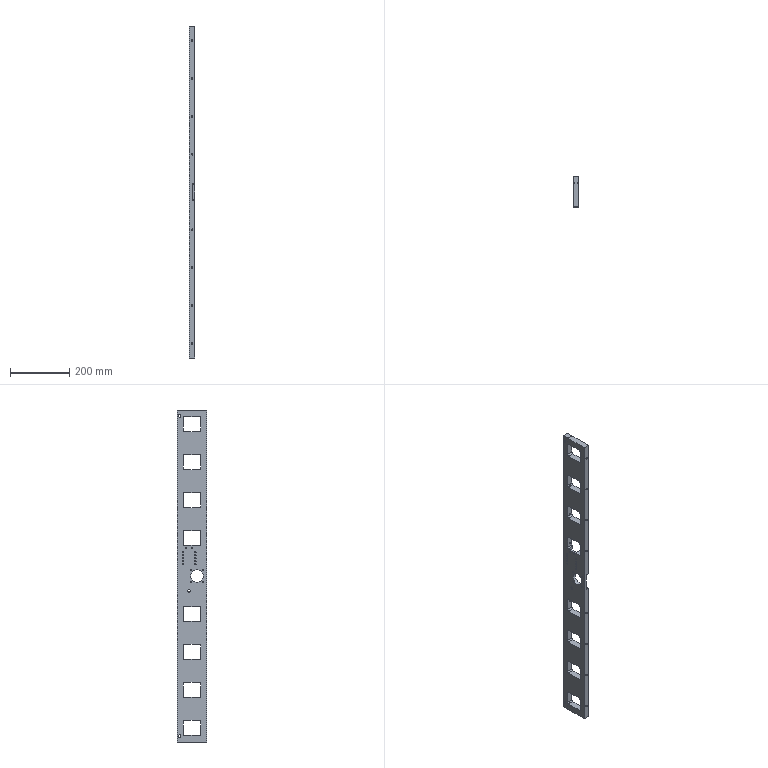Part | NX | 1 solid | 162 faces | box 20 x 100 x 1120 mm | volume 1638064 mm3 | cylinder 91 | plane 53 | cone 18 | commonest cylinder face diameters 10 x38 3.3 x21 4.2 x16 6.5 x8 5 x4 8.5 x3